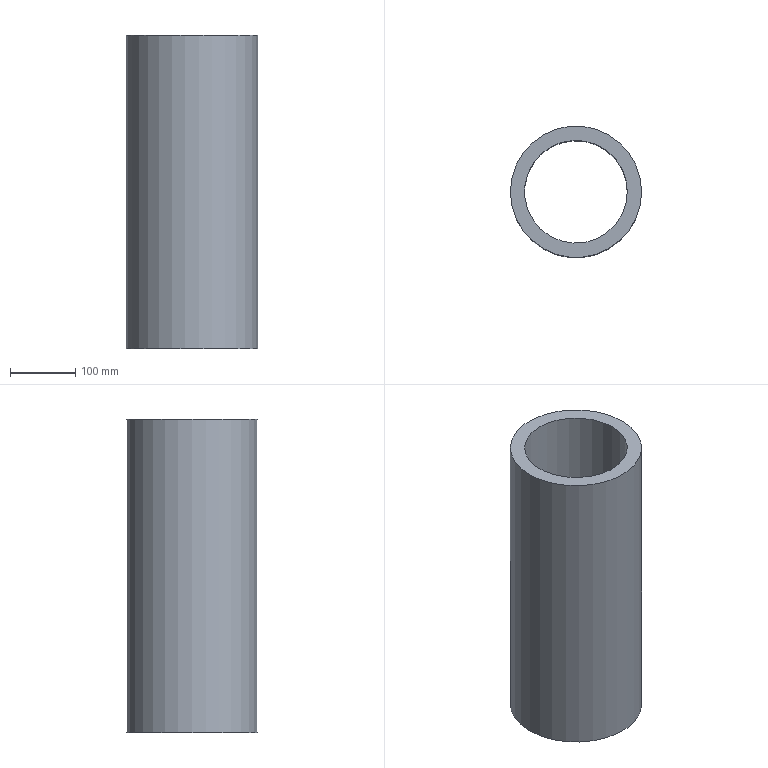Part | NX | features 底座(默认<按焊接>) 2 | 1 solid | 4 faces | box 200.744 x 200.744 x 480 mm | volume 5887277 mm3 | cylinder 2 | plane 2 | commonest cylinder face diameters 157.104 x1 200.744 x1
STEP:
#1=CARTESIAN_POINT('',(1458.357,240.02,480.));
#2=VERTEX_POINT('',#1);
#3=CARTESIAN_POINT('',(1379.805,240.02,480.));
#4=DIRECTION('',(0.,0.,1.));
#5=DIRECTION('',(1.,0.,0.));
#6=AXIS2_PLACEMENT_3D('',#3,#4,#5);
#7=CIRCLE('',#6,78.552);
#8=EDGE_CURVE('',#2,#2,#7,.T.);
#9=ORIENTED_EDGE('',*,*,#8,.T.);
#10=EDGE_LOOP('',(#9));
#11=FACE_BOUND('',#10,.T.);
#12=CARTESIAN_POINT('',(1458.357,240.02,0.));
#13=VERTEX_POINT('',#12);
#14=CARTESIAN_POINT('',(1379.805,240.02,0.));
#15=DIRECTION('',(0.,0.,1.));
#16=DIRECTION('',(1.,0.,0.));
#17=AXIS2_PLACEMENT_3D('',#14,#15,#16);
#18=CIRCLE('',#17,78.552);
#19=EDGE_CURVE('',#13,#13,#18,.T.);
#20=ORIENTED_EDGE('',*,*,#19,.F.);
#21=EDGE_LOOP('',(#20));
#22=FACE_BOUND('',#21,.T.);
#23=CARTESIAN_POINT('',(1379.805,240.02,480.));
#24=DIRECTION('',(0.,0.,-1.));
#25=DIRECTION('',(-1.,0.,0.));
#26=AXIS2_PLACEMENT_3D('',#23,#24,#25);
#27=CYLINDRICAL_SURFACE('',#26,78.552);
#28=ADVANCED_FACE('',(#11,#22),#27,.F.);
#29=CARTESIAN_POINT('',(1480.177,240.02,480.));
#30=VERTEX_POINT('',#29);
#31=CARTESIAN_POINT('',(1379.805,240.02,480.));
#32=DIRECTION('',(0.,0.,1.));
#33=DIRECTION('',(1.,0.,0.));
#34=AXIS2_PLACEMENT_3D('',#31,#32,#33);
#35=CIRCLE('',#34,100.372);
#36=EDGE_CURVE('',#30,#30,#35,.T.);
#37=ORIENTED_EDGE('',*,*,#36,.F.);
#38=EDGE_LOOP('',(#37));
#39=FACE_BOUND('',#38,.T.);
#40=CARTESIAN_POINT('',(1480.177,240.02,0.));
#41=VERTEX_POINT('',#40);
#42=CARTESIAN_POINT('',(1379.805,240.02,0.));
#43=DIRECTION('',(0.,0.,1.));
#44=DIRECTION('',(1.,0.,0.));
#45=AXIS2_PLACEMENT_3D('',#42,#43,#44);
#46=CIRCLE('',#45,100.372);
#47=EDGE_CURVE('',#41,#41,#46,.T.);
#48=ORIENTED_EDGE('',*,*,#47,.T.);
#49=EDGE_LOOP('',(#48));
#50=FACE_BOUND('',#49,.T.);
#51=CARTESIAN_POINT('',(1379.805,240.02,480.));
#52=DIRECTION('',(0.,0.,-1.));
#53=DIRECTION('',(-1.,0.,0.));
#54=AXIS2_PLACEMENT_3D('',#51,#52,#53);
#55=CYLINDRICAL_SURFACE('',#54,100.372);
#56=ADVANCED_FACE('',(#39,#50),#55,.T.);
#57=ORIENTED_EDGE('',*,*,#8,.F.);
#58=EDGE_LOOP('',(#57));
#59=FACE_BOUND('',#58,.T.);
#60=ORIENTED_EDGE('',*,*,#36,.T.);
#61=EDGE_LOOP('',(#60));
#62=FACE_BOUND('',#61,.T.);
#63=CARTESIAN_POINT('',(1250.85,-2373.536,480.));
#64=DIRECTION('',(0.,0.,1.));
#65=DIRECTION('',(1.,0.,0.));
#66=AXIS2_PLACEMENT_3D('',#63,#64,#65);
#67=PLANE('',#66);
#68=ADVANCED_FACE('',(#59,#62),#67,.T.);
#69=ORIENTED_EDGE('',*,*,#19,.T.);
#70=EDGE_LOOP('',(#69));
#71=FACE_BOUND('',#70,.T.);
#72=ORIENTED_EDGE('',*,*,#47,.F.);
#73=EDGE_LOOP('',(#72));
#74=FACE_BOUND('',#73,.T.);
#75=CARTESIAN_POINT('',(1250.85,-2373.536,0.));
#76=DIRECTION('',(0.,0.,1.));
#77=DIRECTION('',(1.,0.,0.));
#78=AXIS2_PLACEMENT_3D('',#75,#76,#77);
#79=PLANE('',#78);
#80=ADVANCED_FACE('',(#71,#74),#79,.F.);
#81=CLOSED_SHELL('',(#28,#56,#68,#80));
#82=MANIFOLD_SOLID_BREP('',#81);
#83=(LENGTH_UNIT()NAMED_UNIT(*)SI_UNIT(.MILLI.,.METRE.));
#84=UNCERTAINTY_MEASURE_WITH_UNIT(LENGTH_MEASURE(0.00001),#83,'','');
#85=(NAMED_UNIT(*)PLANE_ANGLE_UNIT()SI_UNIT($,.RADIAN.));
#86=(NAMED_UNIT(*)SI_UNIT($,.STERADIAN.)SOLID_ANGLE_UNIT());
#87=(GEOMETRIC_REPRESENTATION_CONTEXT(3)GLOBAL_UNCERTAINTY_ASSIGNED_CONTEXT((#84))GLOBAL_UNIT_ASSIGNED_CONTEXT((#83,#85,#86))REPRESENTATION_CONTEXT('',''));
#88=ADVANCED_BREP_SHAPE_REPRESENTATION('',(#82),#87);